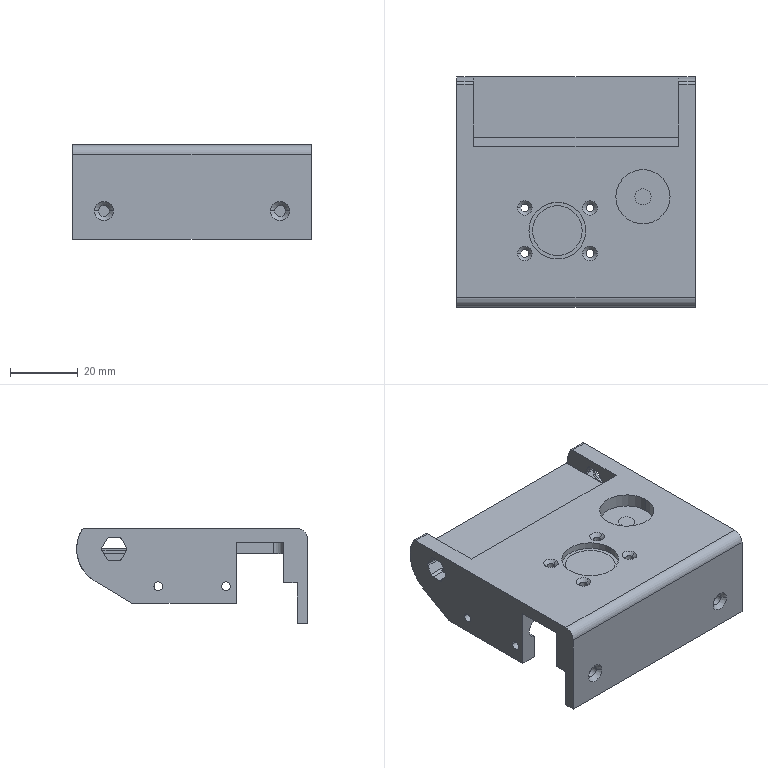NC program | NX | posted with a generic post | part box 70.5 x 68.1 x 28 mm
Lines 654 to 1476 of 2864:
(ZLEVEL_PROFILE_COPY_COPY_1 , TOOL : D2R0.5)
N1288 T09 M6
N1290 G54
N1292 G17 G0 G90 X57.923 Y-3.149 B0. C0. S9500 M3
N1294 G43 Z30. H9
N1296 Z1.
N1298 G94 G1 X57.717 Y-3.082 Z0.989 F1000.
N1300 X57.46 Y-3.043 Z0.975
N1302 X57.229 Y-3.004 Z0.963
N1304 X56.766 Z0.939
N1306 X56.526 Y-3.046 Z0.926
N1308 X56.302 Y-3.076 Z0.914
N1310 X56.048 Y-3.149 Z0.9
N1312 X55.841 Y-3.242 Z0.888
N1314 X55.642 Y-3.322 Z0.877
N1316 X55.312 Y-3.527 Z0.857
N1318 X55.164 Y-3.637 Z0.847
N1320 X55.005 Y-3.749 Z0.837
N1322 X54.966 Y-3.784 Z0.834
N1324 X54.829 Y-3.941 Z0.823
N1326 X54.661 Y-4.116 Z0.81
N1328 X54.308 Y-4.663 Z0.776
N1330 X54.084 Y-5.274 Z0.742
N1332 X54.045 Y-5.519 Z0.729
N1334 X54.027 Y-5.606 Z0.724
N1336 X54.001 Y-6.006 Z0.703
N1338 X54.027 Y-6.394 Z0.683
N1340 X54.046 Y-6.485 Z0.678
N1342 X54.083 Y-6.723 Z0.666
N1344 X54.285 Y-7.292 Z0.634
N1346 X54.601 Y-7.807 Z0.602
N1348 X54.948 Y-8.191 Z0.575
N1350 X55.13 Y-8.355 Z0.562
N1352 X55.236 Y-8.434 Z0.555
N1354 X55.447 Y-8.558 Z0.543
N1356 X55.688 Y-8.693 Z0.528
N1358 X55.9 Y-8.798 Z0.516
N1360 X56.291 Y-8.92 Z0.494
N1362 X56.54 Y-8.957 Z0.481
N1364 X56.771 Y-8.996 Z0.469
N1366 X57.234 Z0.444
N1368 X57.474 Y-8.954 Z0.432
N1370 X57.693 Y-8.926 Z0.42
N1372 X57.959 Y-8.85 Z0.406
N1374 X58.159 Y-8.758 Z0.394
N1376 X58.435 Y-8.629 Z0.378
N1378 X58.745 Y-8.442 Z0.359
N1380 X58.836 Y-8.364 Z0.353
N1382 X59.005 Y-8.24 Z0.342
N1384 X59.021 Y-8.225 Z0.341
N1386 X59.171 Y-8.059 Z0.329
N1388 X59.339 Y-7.884 Z0.316
N1390 X59.692 Y-7.337 Z0.282
N1392 X59.916 Y-6.726 Z0.248
N1394 X59.955 Y-6.481 Z0.235
N1396 X59.973 Y-6.394 Z0.23
N1398 X59.999 Y-6.006 Z0.21
N1400 X59.973 Y-5.606 Z0.189
N1402 X59.954 Y-5.515 Z0.184
N1404 X59.917 Y-5.277 Z0.172
N1406 X59.715 Y-4.708 Z0.14
N1408 X59.399 Y-4.193 Z0.108
N1410 X59.052 Y-3.809 Z0.081
N1412 X58.88 Y-3.651 Z0.069
N1414 X58.856 Y-3.633 Z0.067
N1416 X58.392 Y-3.341 Z0.039
N1418 X58.173 Y-3.229 Z0.026
N1420 X57.717 Y-3.082 Z0.001
N1422 X57.46 Y-3.043 Z-0.013
N1424 X57.229 Y-3.004 Z-0.025
N1426 X56.766 Z-0.05
N1428 X56.526 Y-3.046 Z-0.062
N1430 X56.302 Y-3.076 Z-0.074
N1432 X56.048 Y-3.149 Z-0.088
N1434 X55.841 Y-3.242 Z-0.1
N1436 X55.642 Y-3.322 F1500.
N1438 X55.312 Y-3.527
N1440 X55.164 Y-3.637
N1442 G3 X54.829 Y-3.941 R1.882
N1444 X54.045 Y-5.519 R2.943
N1446 G1 X54.027 Y-5.606
N1448 X54.001 Y-6.006
N1450 X54.027 Y-6.394
N1452 X54.046 Y-6.485
N1454 G3 X54.763 Y-7.986 R2.902
N1456 G1 X54.948 Y-8.191
N1458 G3 X55.447 Y-8.558 R2.996
N1460 G1 X55.688 Y-8.693
N1462 G3 X56.528 Y-8.954 R2.799
N1464 G1 X56.54 Y-8.957
N1466 G3 X57.474 Y-8.954 R2.743
N1468 X58.159 Y-8.758 R2.426
N1470 G1 X58.435 Y-8.629
N1472 X58.644 Y-8.503
N1474 G3 X58.836 Y-8.364 R1.367
N1476 X59.171 Y-8.059 R2.181
N1478 X59.955 Y-6.481 R2.943
N1480 G1 X59.973 Y-6.394
N1482 X59.999 Y-6.006
N1484 X59.973 Y-5.606
N1486 X59.954 Y-5.515
N1488 G3 X59.237 Y-4.014 R2.902
N1490 G1 X59.052 Y-3.809
N1492 G3 X58.658 Y-3.509 R2.717
N1494 G1 X58.392 Y-3.341
N1496 G3 X57.46 Y-3.043 R3.012
N1498 X56.526 Y-3.046 R2.743
N1500 X55.841 Y-3.242 R2.542
N1502 G1 X55.75 Y-3.281 Z-0.102
N1504 X55.66 Y-3.321 Z-0.103
N1506 X55.573 Y-3.367 Z-0.105
N1508 X55.489 Y-3.418 Z-0.107
N1510 X55.404 Y-3.469 Z-0.109
N1512 X55.32 Y-3.52 Z-0.11
N1514 X55.239 Y-3.577 Z-0.112
N1516 X55.161 Y-3.638 Z-0.114
N1518 X55.086 Y-3.702 Z-0.116
N1520 X55.009 Y-3.763 Z-0.117
N1522 X54.935 Y-3.829 Z-0.119
N1524 X54.867 Y-3.901 Z-0.121
N1526 X54.8 Y-3.973 Z-0.122
N1528 X54.732 Y-4.045 Z-0.124
N1530 X54.667 Y-4.119 Z-0.126
N1532 X54.609 Y-4.2 Z-0.128
N1534 X54.552 Y-4.28 Z-0.129
N1536 X54.496 Y-4.361 Z-0.131
N1538 X54.438 Y-4.442 Z-0.133
N1540 X54.393 Y-4.53 Z-0.134
N1542 X54.347 Y-4.617 Z-0.136
N1544 X54.302 Y-4.705 Z-0.138
N1546 X54.257 Y-4.793 Z-0.14
N1548 X54.222 Y-4.885 Z-0.141
N1550 X54.188 Y-4.978 Z-0.143
N1552 X54.155 Y-5.071 Z-0.145
N1554 X54.123 Y-5.164 Z-0.147
N1556 X54.099 Y-5.26 Z-0.148
N1558 X54.079 Y-5.357 Z-0.15
N1560 X54.059 Y-5.453 Z-0.152
N1562 X54.039 Y-5.55 Z-0.153
N1564 X54.026 Y-5.648 Z-0.155
N1566 X54.019 Y-5.746 Z-0.157
N1568 X54.013 Y-5.845 Z-0.159
N1570 X54.006 Y-5.943 Z-0.16
N1572 X54.003 Y-6.042 Z-0.162
N1574 X54.011 Y-6.14 Z-0.164
N1576 X54.018 Y-6.239 Z-0.166
N1578 X54.025 Y-6.337 Z-0.167
N1580 X54.035 Y-6.436 Z-0.169
N1582 X54.055 Y-6.532 Z-0.171
N1584 X54.076 Y-6.629 Z-0.172
N1586 X54.096 Y-6.725 Z-0.174
N1588 X54.117 Y-6.822 Z-0.176
N1590 X54.15 Y-6.915 Z-0.178
N1592 X54.184 Y-7.008 Z-0.179
N1594 X54.217 Y-7.101 Z-0.181
N1596 X54.25 Y-7.194 Z-0.183
N1598 X54.295 Y-7.282 Z-0.184
N1600 X54.341 Y-7.369 Z-0.186
N1602 X54.386 Y-7.457 Z-0.188
N1604 X54.431 Y-7.545 Z-0.19
N1606 X54.487 Y-7.627 Z-0.191
N1608 X54.544 Y-7.707 Z-0.193
N1610 X54.6 Y-7.788 Z-0.195
N1612 X54.658 Y-7.869 Z-0.197
N1614 X54.722 Y-7.943 Z-0.198
N1616 X54.79 Y-8.016 Z-0.2
N1618 X54.949 Y-8.191
N1620 G3 X55.447 Y-8.558 R2.994
N1622 G1 X55.688 Y-8.693
N1624 G3 X56.528 Y-8.954 R2.798
N1626 G1 X56.54 Y-8.957
N1628 G3 X57.474 Y-8.954 R2.743
N1630 X58.159 Y-8.758 R2.431
N1632 G1 X58.433 Y-8.63
N1634 X58.644 Y-8.503
N1636 G3 X58.836 Y-8.364 R1.367
N1638 X59.171 Y-8.059 R2.181
N1640 X59.955 Y-6.481 R2.943
N1642 G1 X59.973 Y-6.394
N1644 X59.999 Y-6.006
N1646 X59.973 Y-5.606
N1648 X59.954 Y-5.515
N1650 G3 X59.236 Y-4.013 R2.903
N1652 G1 X59.051 Y-3.809
N1654 G3 X58.659 Y-3.509 R2.714
N1656 G1 X58.392 Y-3.341
N1658 G3 X57.46 Y-3.043 R3.013
N1660 X56.526 Y-3.046 R2.743
N1662 X55.841 Y-3.242 R2.542
N1664 G1 X55.75 Y-3.281 Z-0.202
N1666 X55.66 Y-3.321 Z-0.203
N1668 X55.573 Y-3.367 Z-0.205
N1670 X55.489 Y-3.418 Z-0.207
N1672 X55.404 Y-3.469 Z-0.209
N1674 X55.32 Y-3.52 Z-0.21
N1676 X55.239 Y-3.577 Z-0.212
N1678 X55.161 Y-3.638 Z-0.214
N1680 X55.086 Y-3.701 Z-0.216
N1682 X55.009 Y-3.763 Z-0.217
N1684 X54.935 Y-3.829 Z-0.219
N1686 X54.867 Y-3.901 Z-0.221
N1688 X54.8 Y-3.973 Z-0.222
N1690 X54.732 Y-4.045 Z-0.224
N1692 X54.667 Y-4.119 Z-0.226
N1694 X54.609 Y-4.2 Z-0.228
N1696 X54.552 Y-4.28 Z-0.229
N1698 X54.496 Y-4.361 Z-0.231
N1700 X54.438 Y-4.442 Z-0.233
N1702 X54.393 Y-4.53 Z-0.234
N1704 X54.347 Y-4.617 Z-0.236
N1706 X54.302 Y-4.705 Z-0.238
N1708 X54.257 Y-4.793 Z-0.24
N1710 X54.222 Y-4.885 Z-0.241
N1712 X54.188 Y-4.978 Z-0.243
N1714 X54.155 Y-5.071 Z-0.245
N1716 X54.123 Y-5.164 Z-0.247
N1718 X54.099 Y-5.26 Z-0.248
N1720 X54.079 Y-5.357 Z-0.25
N1722 X54.059 Y-5.453 Z-0.252
N1724 X54.039 Y-5.55 Z-0.253
N1726 X54.026 Y-5.648 Z-0.255
N1728 X54.019 Y-5.746 Z-0.257
N1730 X54.013 Y-5.845 Z-0.259
N1732 X54.006 Y-5.943 Z-0.26
N1734 X54.003 Y-6.042 Z-0.262
N1736 X54.011 Y-6.14 Z-0.264
N1738 X54.018 Y-6.239 Z-0.266
N1740 X54.025 Y-6.337 Z-0.267
N1742 X54.035 Y-6.436 Z-0.269
N1744 X54.055 Y-6.532 Z-0.271
N1746 X54.076 Y-6.629 Z-0.272
N1748 X54.096 Y-6.725 Z-0.274
N1750 X54.117 Y-6.822 Z-0.276
N1752 X54.15 Y-6.915 Z-0.278
N1754 X54.184 Y-7.008 Z-0.279
N1756 X54.217 Y-7.101 Z-0.281
N1758 X54.25 Y-7.194 Z-0.283
N1760 X54.295 Y-7.282 Z-0.284
N1762 X54.34 Y-7.369 Z-0.286
N1764 X54.386 Y-7.457 Z-0.288
N1766 X54.431 Y-7.545 Z-0.29
N1768 X54.487 Y-7.627 Z-0.291
N1770 X54.544 Y-7.707 Z-0.293
N1772 X54.6 Y-7.788 Z-0.295
N1774 X54.658 Y-7.869 Z-0.297
N1776 X54.722 Y-7.943 Z-0.298
N1778 X54.79 Y-8.016 Z-0.3
N1780 X54.949 Y-8.191
N1782 G3 X55.447 Y-8.558 R2.993
N1784 G1 X55.689 Y-8.694
N1786 G3 X56.528 Y-8.954 R2.797
N1788 G1 X56.54 Y-8.957
N1790 G3 X57.474 Y-8.954 R2.743
N1792 X58.159 Y-8.758 R2.436
N1794 G1 X58.431 Y-8.631
N1796 X58.644 Y-8.503
N1798 G3 X58.836 Y-8.364 R1.367
N1800 X59.171 Y-8.059 R2.181
N1802 X59.955 Y-6.481 R2.943
N1804 G1 X59.973 Y-6.394
N1806 X59.999 Y-6.006
N1808 X59.973 Y-5.606
N1810 X59.954 Y-5.515
N1812 G3 X59.236 Y-4.012 R2.903
N1814 G1 X59.051 Y-3.809
N1816 G3 X58.659 Y-3.509 R2.712
N1818 G1 X58.392 Y-3.341
N1820 G3 X57.46 Y-3.043 R3.013
N1822 X56.526 Y-3.046 R2.743
N1824 X55.841 Y-3.242 R2.542
N1826 G1 X55.75 Y-3.281 Z-0.302
N1828 X55.66 Y-3.321 Z-0.303
N1830 X55.573 Y-3.367 Z-0.305
N1832 X55.489 Y-3.418 Z-0.307
N1834 X55.404 Y-3.469 Z-0.309
N1836 X55.32 Y-3.52 Z-0.31
N1838 X55.239 Y-3.577 Z-0.312
N1840 X55.161 Y-3.638 Z-0.314
N1842 X55.085 Y-3.701 Z-0.316
N1844 X55.009 Y-3.764 Z-0.317
N1846 X54.935 Y-3.829 Z-0.319
N1848 X54.867 Y-3.901 Z-0.321
N1850 X54.8 Y-3.973 Z-0.322
N1852 X54.732 Y-4.045 Z-0.324
N1854 X54.667 Y-4.119 Z-0.326
N1856 X54.609 Y-4.2 Z-0.328
N1858 X54.552 Y-4.28 Z-0.329
N1860 X54.496 Y-4.361 Z-0.331
N1862 X54.438 Y-4.442 Z-0.333
N1864 X54.393 Y-4.53 Z-0.334
N1866 X54.347 Y-4.617 Z-0.336
N1868 X54.302 Y-4.705 Z-0.338
N1870 X54.257 Y-4.793 Z-0.34
N1872 X54.222 Y-4.885 Z-0.341
N1874 X54.188 Y-4.978 Z-0.343
N1876 X54.155 Y-5.071 Z-0.345
N1878 X54.123 Y-5.164 Z-0.347
N1880 X54.099 Y-5.26 Z-0.348
N1882 X54.079 Y-5.357 Z-0.35
N1884 X54.059 Y-5.453 Z-0.352
N1886 X54.039 Y-5.55 Z-0.353
N1888 X54.026 Y-5.648 Z-0.355
N1890 X54.019 Y-5.746 Z-0.357
N1892 X54.013 Y-5.845 Z-0.359
N1894 X54.006 Y-5.943 Z-0.36
N1896 X54.003 Y-6.042 Z-0.362
N1898 X54.011 Y-6.14 Z-0.364
N1900 X54.018 Y-6.239 Z-0.366
N1902 X54.025 Y-6.337 Z-0.367
N1904 X54.035 Y-6.436 Z-0.369
N1906 X54.055 Y-6.532 Z-0.371
N1908 X54.076 Y-6.629 Z-0.372
N1910 X54.096 Y-6.725 Z-0.374
N1912 X54.117 Y-6.822 Z-0.376
N1914 X54.15 Y-6.915 Z-0.378
N1916 X54.184 Y-7.008 Z-0.379
N1918 X54.217 Y-7.101 Z-0.381
N1920 X54.25 Y-7.194 Z-0.383
N1922 X54.295 Y-7.282 Z-0.384
N1924 X54.34 Y-7.369 Z-0.386
N1926 X54.386 Y-7.457 Z-0.388
N1928 X54.431 Y-7.545 Z-0.39
N1930 X54.487 Y-7.627 Z-0.391
N1932 X54.544 Y-7.707 Z-0.393
N1934 X54.6 Y-7.788 Z-0.395
N1936 X54.658 Y-7.869 Z-0.397
N1938 X54.722 Y-7.943 Z-0.398
N1940 X54.79 Y-8.016 Z-0.4
N1942 X54.949 Y-8.191
N1944 G3 X55.447 Y-8.558 R2.991
N1946 G1 X55.689 Y-8.694
N1948 G3 X56.528 Y-8.954 R2.795
N1950 G1 X56.54 Y-8.957
N1952 G3 X57.474 Y-8.954 R2.743
N1954 X58.159 Y-8.758 R2.441
N1956 G1 X58.429 Y-8.632
N1958 X58.644 Y-8.503
N1960 G3 X58.836 Y-8.364 R1.367
N1962 X59.171 Y-8.059 R2.181
N1964 X59.955 Y-6.481 R2.943
N1966 G1 X59.973 Y-6.394
N1968 X59.999 Y-6.006
N1970 X59.973 Y-5.606
N1972 X59.954 Y-5.515
N1974 G3 X59.235 Y-4.012 R2.904
N1976 G1 X59.051 Y-3.809
N1978 G3 X58.659 Y-3.509 R2.71
N1980 G1 X58.392 Y-3.341
N1982 G3 X57.46 Y-3.043 R3.013
N1984 X56.526 Y-3.046 R2.743
N1986 X55.841 Y-3.242 R2.542
N1988 G1 X55.75 Y-3.281 Z-0.402
N1990 X55.66 Y-3.321 Z-0.403
N1992 X55.573 Y-3.367 Z-0.405
N1994 X55.489 Y-3.418 Z-0.407
N1996 X55.404 Y-3.469 Z-0.409
N1998 X55.32 Y-3.52 Z-0.41
N2000 X55.239 Y-3.577 Z-0.412
N2002 X55.162 Y-3.639 Z-0.414
N2004 X55.085 Y-3.701 Z-0.416
N2006 X55.009 Y-3.764 Z-0.417
N2008 X54.935 Y-3.829 Z-0.419
N2010 X54.867 Y-3.901 Z-0.421
N2012 X54.8 Y-3.973 Z-0.422
N2014 X54.733 Y-4.045 Z-0.424
N2016 X54.666 Y-4.119 Z-0.426
N2018 X54.61 Y-4.2 Z-0.428
N2020 X54.553 Y-4.28 Z-0.429
N2022 X54.496 Y-4.361 Z-0.431
N2024 X54.438 Y-4.442 Z-0.433
N2026 X54.393 Y-4.53 Z-0.434
N2028 X54.348 Y-4.617 Z-0.436
N2030 X54.303 Y-4.705 Z-0.438
N2032 X54.257 Y-4.793 Z-0.44
N2034 X54.221 Y-4.885 Z-0.441
N2036 X54.189 Y-4.978 Z-0.443
N2038 X54.156 Y-5.071 Z-0.445
N2040 X54.122 Y-5.164 Z-0.447
N2042 X54.099 Y-5.26 Z-0.448
N2044 X54.079 Y-5.357 Z-0.45
N2046 X54.059 Y-5.453 Z-0.452
N2048 X54.039 Y-5.55 Z-0.453
N2050 X54.026 Y-5.648 Z-0.455
N2052 X54.019 Y-5.746 Z-0.457
N2054 X54.013 Y-5.845 Z-0.459
N2056 X54.006 Y-5.943 Z-0.46
N2058 X54.004 Y-6.042 Z-0.462
N2060 X54.011 Y-6.14 Z-0.464
N2062 X54.017 Y-6.239 Z-0.466
N2064 X54.025 Y-6.337 Z-0.467
N2066 X54.036 Y-6.435 Z-0.469
N2068 X54.055 Y-6.532 Z-0.471
N2070 X54.076 Y-6.629 Z-0.472
N2072 X54.096 Y-6.725 Z-0.474
N2074 X54.117 Y-6.822 Z-0.476
N2076 X54.15 Y-6.915 Z-0.478
N2078 X54.184 Y-7.008 Z-0.479
N2080 X54.217 Y-7.101 Z-0.481
N2082 X54.25 Y-7.194 Z-0.483
N2084 X54.295 Y-7.282 Z-0.484
N2086 X54.341 Y-7.369 Z-0.486
N2088 X54.386 Y-7.457 Z-0.488
N2090 X54.431 Y-7.545 Z-0.49
N2092 X54.487 Y-7.626 Z-0.491
N2094 X54.544 Y-7.707 Z-0.493
N2096 X54.601 Y-7.788 Z-0.495
N2098 X54.658 Y-7.869 Z-0.497
N2100 X54.722 Y-7.944 Z-0.498
N2102 X54.783 Y-8.022 Z-0.5
N2104 G3 X55.838 Y-3.234 R-3.
N2106 G1 X55.747 Y-3.274 Z-0.502
N2108 X55.658 Y-3.317 Z-0.503
N2110 X55.571 Y-3.362 Z-0.505
N2112 X55.484 Y-3.411 Z-0.507
N2114 X55.4 Y-3.462 Z-0.509
N2116 X55.317 Y-3.516 Z-0.51
N2118 X55.237 Y-3.573 Z-0.512
N2120 X55.158 Y-3.632 Z-0.514
N2122 X55.081 Y-3.694 Z-0.516
N2124 X55.006 Y-3.759 Z-0.517
N2126 X54.933 Y-3.826 Z-0.519
N2128 X54.863 Y-3.895 Z-0.521
N2130 X54.795 Y-3.966 Z-0.522
N2132 X54.729 Y-4.04 Z-0.524
N2134 X54.665 Y-4.116 Z-0.526
N2136 X54.605 Y-4.194 Z-0.528
N2138 X54.547 Y-4.274 Z-0.529
N2140 X54.491 Y-4.355 Z-0.531
N2142 X54.438 Y-4.439 Z-0.533
N2144 X54.388 Y-4.524 Z-0.534
N2146 X54.341 Y-4.611 Z-0.536
N2148 X54.297 Y-4.699 Z-0.538
N2150 X54.255 Y-4.789 Z-0.54
N2152 X54.217 Y-4.88 Z-0.541
N2154 X54.182 Y-4.972 Z-0.543
N2156 X54.149 Y-5.065 Z-0.545
N2158 X54.12 Y-5.16 Z-0.547
N2160 X54.094 Y-5.255 Z-0.548
N2162 X54.071 Y-5.351 Z-0.55
N2164 X54.051 Y-5.448 Z-0.552
N2166 X54.035 Y-5.545 Z-0.553
N2168 X54.021 Y-5.643 Z-0.555
N2170 X54.011 Y-5.741 Z-0.557
N2172 X54.004 Y-5.84 Z-0.559
N2174 X54.001 Y-5.938 Z-0.56
N2176 X54. Y-6.037 Z-0.562
N2178 X54.003 Y-6.136 Z-0.564
N2180 X54.009 Y-6.234 Z-0.566
N2182 X54.019 Y-6.333 Z-0.567
N2184 X54.031 Y-6.431 Z-0.569
N2186 X54.047 Y-6.528 Z-0.571
N2188 X54.066 Y-6.625 Z-0.572
N2190 X54.088 Y-6.721 Z-0.574
N2192 X54.113 Y-6.817 Z-0.576
N2194 X54.142 Y-6.912 Z-0.578
N2196 X54.173 Y-7.005 Z-0.579
N2198 X54.208 Y-7.098 Z-0.581
N2200 X54.246 Y-7.189 Z-0.583
N2202 X54.286 Y-7.279 Z-0.584
N2204 X54.33 Y-7.368 Z-0.586
N2206 X54.376 Y-7.455 Z-0.588
N2208 X54.426 Y-7.54 Z-0.59
N2210 X54.478 Y-7.624 Z-0.591
N2212 X54.533 Y-7.706 Z-0.593
N2214 X54.59 Y-7.787 Z-0.595
N2216 X54.65 Y-7.865 Z-0.597
N2218 X54.713 Y-7.941 Z-0.598
N2220 X54.778 Y-8.016 Z-0.6
N2222 G3 X55.838 Y-3.234 R-3.
N2224 G1 X55.747 Y-3.274 Z-0.602
N2226 X55.658 Y-3.317 Z-0.603
N2228 X55.571 Y-3.362 Z-0.605
N2230 X55.484 Y-3.411 Z-0.607
N2232 X55.4 Y-3.462 Z-0.609
N2234 X55.317 Y-3.516 Z-0.61
N2236 X55.237 Y-3.573 Z-0.612
N2238 X55.158 Y-3.632 Z-0.614
N2240 X55.081 Y-3.694 Z-0.616
N2242 X55.006 Y-3.759 Z-0.617
N2244 X54.933 Y-3.826 Z-0.619
N2246 X54.863 Y-3.895 Z-0.621
N2248 X54.795 Y-3.966 Z-0.622
N2250 X54.729 Y-4.04 Z-0.624
N2252 X54.665 Y-4.116 Z-0.626
N2254 X54.605 Y-4.194 Z-0.628
N2256 X54.547 Y-4.274 Z-0.629
N2258 X54.491 Y-4.355 Z-0.631
N2260 X54.438 Y-4.439 Z-0.633
N2262 X54.388 Y-4.524 Z-0.634
N2264 X54.341 Y-4.611 Z-0.636
N2266 X54.297 Y-4.699 Z-0.638
N2268 X54.255 Y-4.789 Z-0.64
N2270 X54.217 Y-4.88 Z-0.641
N2272 X54.182 Y-4.972 Z-0.643
N2274 X54.149 Y-5.065 Z-0.645
N2276 X54.12 Y-5.16 Z-0.647
N2278 X54.094 Y-5.255 Z-0.648
N2280 X54.071 Y-5.351 Z-0.65
N2282 X54.051 Y-5.448 Z-0.652
N2284 X54.035 Y-5.545 Z-0.653
N2286 X54.021 Y-5.643 Z-0.655
N2288 X54.011 Y-5.741 Z-0.657
N2290 X54.004 Y-5.84 Z-0.659
N2292 X54.001 Y-5.938 Z-0.66
N2294 X54. Y-6.037 Z-0.662
N2296 X54.003 Y-6.136 Z-0.664
N2298 X54.009 Y-6.234 Z-0.666
N2300 X54.019 Y-6.333 Z-0.667
N2302 X54.031 Y-6.431 Z-0.669
N2304 X54.047 Y-6.528 Z-0.671
N2306 X54.066 Y-6.625 Z-0.672
N2308 X54.088 Y-6.721 Z-0.674
N2310 X54.113 Y-6.817 Z-0.676
N2312 X54.142 Y-6.912 Z-0.678
N2314 X54.173 Y-7.005 Z-0.679
N2316 X54.208 Y-7.098 Z-0.681
N2318 X54.246 Y-7.189 Z-0.683
N2320 X54.286 Y-7.279 Z-0.684
N2322 X54.33 Y-7.368 Z-0.686
N2324 X54.376 Y-7.455 Z-0.688
N2326 X54.426 Y-7.54 Z-0.69
N2328 X54.478 Y-7.624 Z-0.691
N2330 X54.533 Y-7.706 Z-0.693
N2332 X54.59 Y-7.787 Z-0.695
N2334 X54.65 Y-7.865 Z-0.697
N2336 X54.713 Y-7.941 Z-0.698
N2338 X54.778 Y-8.016 Z-0.7
N2340 G3 X55.838 Y-3.234 R-3.
N2342 G1 X55.747 Y-3.274 Z-0.702
N2344 X55.658 Y-3.317 Z-0.703
N2346 X55.571 Y-3.362 Z-0.705
N2348 X55.484 Y-3.411 Z-0.707
N2350 X55.4 Y-3.462 Z-0.709
N2352 X55.317 Y-3.516 Z-0.71
N2354 X55.237 Y-3.573 Z-0.712
N2356 X55.158 Y-3.632 Z-0.714
N2358 X55.081 Y-3.694 Z-0.716
N2360 X55.006 Y-3.759 Z-0.717
N2362 X54.933 Y-3.826 Z-0.719
N2364 X54.863 Y-3.895 Z-0.721
N2366 X54.795 Y-3.966 Z-0.722
N2368 X54.729 Y-4.04 Z-0.724
N2370 X54.665 Y-4.116 Z-0.726
N2372 X54.605 Y-4.194 Z-0.728
N2374 X54.547 Y-4.274 Z-0.729
N2376 X54.491 Y-4.355 Z-0.731
N2378 X54.438 Y-4.439 Z-0.733
N2380 X54.388 Y-4.524 Z-0.734
N2382 X54.341 Y-4.611 Z-0.736
N2384 X54.297 Y-4.699 Z-0.738
N2386 X54.255 Y-4.789 Z-0.74
N2388 X54.217 Y-4.88 Z-0.741
N2390 X54.182 Y-4.972 Z-0.743
N2392 X54.149 Y-5.065 Z-0.745
N2394 X54.12 Y-5.16 Z-0.747
N2396 X54.094 Y-5.255 Z-0.748
N2398 X54.071 Y-5.351 Z-0.75
N2400 X54.051 Y-5.448 Z-0.752
N2402 X54.035 Y-5.545 Z-0.753
N2404 X54.021 Y-5.643 Z-0.755
N2406 X54.011 Y-5.741 Z-0.757
N2408 X54.004 Y-5.84 Z-0.759
N2410 X54.001 Y-5.938 Z-0.76
N2412 X54. Y-6.037 Z-0.762
N2414 X54.003 Y-6.136 Z-0.764
N2416 X54.009 Y-6.234 Z-0.766
N2418 X54.019 Y-6.333 Z-0.767
N2420 X54.031 Y-6.431 Z-0.769
N2422 X54.047 Y-6.528 Z-0.771
N2424 X54.066 Y-6.625 Z-0.772
N2426 X54.088 Y-6.721 Z-0.774
N2428 X54.113 Y-6.817 Z-0.776
N2430 X54.142 Y-6.912 Z-0.778
N2432 X54.173 Y-7.005 Z-0.779
N2434 X54.208 Y-7.098 Z-0.781
N2436 X54.246 Y-7.189 Z-0.783
N2438 X54.286 Y-7.279 Z-0.784
N2440 X54.33 Y-7.368 Z-0.786
N2442 X54.376 Y-7.455 Z-0.788
N2444 X54.426 Y-7.54 Z-0.79
N2446 X54.478 Y-7.624 Z-0.791
N2448 X54.533 Y-7.706 Z-0.793
N2450 X54.59 Y-7.787 Z-0.795
N2452 X54.65 Y-7.865 Z-0.797
N2454 X54.713 Y-7.941 Z-0.798
N2456 X54.778 Y-8.016 Z-0.8
N2458 G3 X55.838 Y-3.234 R-3.
N2460 G1 X55.747 Y-3.274 Z-0.802
N2462 X55.658 Y-3.317 Z-0.803
N2464 X55.571 Y-3.362 Z-0.805
N2466 X55.484 Y-3.411 Z-0.807
N2468 X55.4 Y-3.462 Z-0.809
N2470 X55.317 Y-3.516 Z-0.81
N2472 X55.237 Y-3.573 Z-0.812
N2474 X55.158 Y-3.632 Z-0.814
N2476 X55.081 Y-3.694 Z-0.816
N2478 X55.006 Y-3.759 Z-0.817
N2480 X54.933 Y-3.826 Z-0.819
N2482 X54.863 Y-3.895 Z-0.821
N2484 X54.795 Y-3.966 Z-0.822
N2486 X54.729 Y-4.04 Z-0.824
N2488 X54.665 Y-4.116 Z-0.826
N2490 X54.605 Y-4.194 Z-0.828
N2492 X54.547 Y-4.274 Z-0.829
N2494 X54.491 Y-4.355 Z-0.831
N2496 X54.438 Y-4.439 Z-0.833
N2498 X54.388 Y-4.524 Z-0.834
N2500 X54.341 Y-4.611 Z-0.836
N2502 X54.297 Y-4.699 Z-0.838
N2504 X54.255 Y-4.789 Z-0.84
N2506 X54.217 Y-4.88 Z-0.841
N2508 X54.182 Y-4.972 Z-0.843
N2510 X54.149 Y-5.065 Z-0.845
N2512 X54.12 Y-5.16 Z-0.847
N2514 X54.094 Y-5.255 Z-0.848
N2516 X54.071 Y-5.351 Z-0.85
N2518 X54.051 Y-5.448 Z-0.852
N2520 X54.035 Y-5.545 Z-0.853
N2522 X54.021 Y-5.643 Z-0.855
N2524 X54.011 Y-5.741 Z-0.857
N2526 X54.004 Y-5.84 Z-0.859
N2528 X54.001 Y-5.938 Z-0.86
N2530 X54. Y-6.037 Z-0.862
N2532 X54.003 Y-6.136 Z-0.864
N2534 X54.009 Y-6.234 Z-0.866
N2536 X54.019 Y-6.333 Z-0.867
N2538 X54.031 Y-6.431 Z-0.869
N2540 X54.047 Y-6.528 Z-0.871
N2542 X54.066 Y-6.625 Z-0.872
N2544 X54.088 Y-6.721 Z-0.874
N2546 X54.113 Y-6.817 Z-0.876
N2548 X54.142 Y-6.912 Z-0.878
N2550 X54.173 Y-7.005 Z-0.879
N2552 X54.208 Y-7.098 Z-0.881
N2554 X54.246 Y-7.189 Z-0.883
N2556 X54.286 Y-7.279 Z-0.884
N2558 X54.33 Y-7.368 Z-0.886
N2560 X54.376 Y-7.455 Z-0.888
N2562 X54.426 Y-7.54 Z-0.89
N2564 X54.478 Y-7.624 Z-0.891
N2566 X54.533 Y-7.706 Z-0.893
N2568 X54.59 Y-7.787 Z-0.895
N2570 X54.65 Y-7.865 Z-0.897
N2572 X54.713 Y-7.941 Z-0.898
N2574 X54.778 Y-8.016 Z-0.9
N2576 G3 X55.838 Y-3.234 R-3.
N2578 G1 X55.747 Y-3.274 Z-0.902
N2580 X55.658 Y-3.317 Z-0.903
N2582 X55.571 Y-3.362 Z-0.905
N2584 X55.484 Y-3.411 Z-0.907
N2586 X55.4 Y-3.462 Z-0.909
N2588 X55.317 Y-3.516 Z-0.91
N2590 X55.237 Y-3.573 Z-0.912
N2592 X55.158 Y-3.632 Z-0.914
N2594 X55.081 Y-3.694 Z-0.916
N2596 X55.006 Y-3.759 Z-0.917
N2598 X54.933 Y-3.826 Z-0.919
N2600 X54.863 Y-3.895 Z-0.921
N2602 X54.795 Y-3.966 Z-0.922
N2604 X54.729 Y-4.04 Z-0.924
N2606 X54.665 Y-4.116 Z-0.926
N2608 X54.605 Y-4.194 Z-0.928
N2610 X54.547 Y-4.274 Z-0.929
N2612 X54.491 Y-4.355 Z-0.931
N2614 X54.438 Y-4.439 Z-0.933
N2616 X54.388 Y-4.524 Z-0.934
N2618 X54.341 Y-4.611 Z-0.936
N2620 X54.297 Y-4.699 Z-0.938
N2622 X54.255 Y-4.789 Z-0.94
N2624 X54.217 Y-4.88 Z-0.941
N2626 X54.182 Y-4.972 Z-0.943
N2628 X54.149 Y-5.065 Z-0.945
N2630 X54.12 Y-5.16 Z-0.947
N2632 X54.094 Y-5.255 Z-0.948
N2634 X54.071 Y-5.351 Z-0.95
N2636 X54.051 Y-5.448 Z-0.952
N2638 X54.035 Y-5.545 Z-0.953
N2640 X54.021 Y-5.643 Z-0.955
N2642 X54.011 Y-5.741 Z-0.957
N2644 X54.004 Y-5.84 Z-0.959
N2646 X54.001 Y-5.938 Z-0.96
N2648 X54. Y-6.037 Z-0.962
N2650 X54.003 Y-6.136 Z-0.964
N2652 X54.009 Y-6.234 Z-0.966
N2654 X54.019 Y-6.333 Z-0.967
N2656 X54.031 Y-6.431 Z-0.969
N2658 X54.047 Y-6.528 Z-0.971
N2660 X54.066 Y-6.625 Z-0.972
N2662 X54.088 Y-6.721 Z-0.974
N2664 X54.113 Y-6.817 Z-0.976
N2666 X54.142 Y-6.912 Z-0.978
N2668 X54.173 Y-7.005 Z-0.979
N2670 X54.208 Y-7.098 Z-0.981
N2672 X54.246 Y-7.189 Z-0.983
N2674 X54.286 Y-7.279 Z-0.984
N2676 X54.33 Y-7.368 Z-0.986
N2678 X54.376 Y-7.455 Z-0.988
N2680 X54.426 Y-7.54 Z-0.99
N2682 X54.478 Y-7.624 Z-0.991
N2684 X54.533 Y-7.706 Z-0.993
N2686 X54.59 Y-7.787 Z-0.995
N2688 X54.65 Y-7.865 Z-0.997
N2690 X54.713 Y-7.941 Z-0.998
N2692 X54.778 Y-8.016 Z-1.
N2694 G3 X55.838 Y-3.234 R-3.
N2696 G1 X55.747 Y-3.274 Z-1.002
N2698 X55.658 Y-3.317 Z-1.003
N2700 X55.571 Y-3.362 Z-1.005
N2702 X55.484 Y-3.411 Z-1.007
N2704 X55.4 Y-3.462 Z-1.009
N2706 X55.317 Y-3.516 Z-1.01
N2708 X55.237 Y-3.573 Z-1.012
N2710 X55.158 Y-3.632 Z-1.014
N2712 X55.081 Y-3.694 Z-1.016
N2714 X55.006 Y-3.759 Z-1.017
N2716 X54.933 Y-3.826 Z-1.019
N2718 X54.863 Y-3.895 Z-1.021
N2720 X54.795 Y-3.966 Z-1.022
N2722 X54.729 Y-4.04 Z-1.024
N2724 X54.665 Y-4.116 Z-1.026
N2726 X54.605 Y-4.194 Z-1.028
N2728 X54.547 Y-4.274 Z-1.029
N2730 X54.491 Y-4.355 Z-1.031
N2732 X54.438 Y-4.439 Z-1.033
N2734 X54.388 Y-4.524 Z-1.034
N2736 X54.341 Y-4.611 Z-1.036
N2738 X54.297 Y-4.699 Z-1.038
N2740 X54.255 Y-4.789 Z-1.04
N2742 X54.217 Y-4.88 Z-1.041
N2744 X54.182 Y-4.972 Z-1.043
N2746 X54.149 Y-5.065 Z-1.045
N2748 X54.12 Y-5.16 Z-1.047
N2750 X54.094 Y-5.255 Z-1.048
N2752 X54.071 Y-5.351 Z-1.05
N2754 X54.051 Y-5.448 Z-1.052
N2756 X54.035 Y-5.545 Z-1.053
N2758 X54.021 Y-5.643 Z-1.055
N2760 X54.011 Y-5.741 Z-1.057
N2762 X54.004 Y-5.84 Z-1.059
N2764 X54.001 Y-5.938 Z-1.06
N2766 X54. Y-6.037 Z-1.062
N2768 X54.003 Y-6.136 Z-1.064
N2770 X54.009 Y-6.234 Z-1.066
N2772 X54.019 Y-6.333 Z-1.067
N2774 X54.031 Y-6.431 Z-1.069
N2776 X54.047 Y-6.528 Z-1.071
N2778 X54.066 Y-6.625 Z-1.072
N2780 X54.088 Y-6.721 Z-1.074
N2782 X54.113 Y-6.817 Z-1.076
N2784 X54.142 Y-6.912 Z-1.078
N2786 X54.173 Y-7.005 Z-1.079
N2788 X54.208 Y-7.098 Z-1.081
N2790 X54.246 Y-7.189 Z-1.083
N2792 X54.286 Y-7.279 Z-1.084
N2794 X54.33 Y-7.368 Z-1.086
N2796 X54.376 Y-7.455 Z-1.088
N2798 X54.426 Y-7.54 Z-1.09
N2800 X54.478 Y-7.624 Z-1.091
N2802 X54.533 Y-7.706 Z-1.093
N2804 X54.59 Y-7.787 Z-1.095
N2806 X54.65 Y-7.865 Z-1.097
N2808 X54.713 Y-7.941 Z-1.098
N2810 X54.778 Y-8.016 Z-1.1
N2812 G3 X55.838 Y-3.234 R-3.
N2814 G1 X55.747 Y-3.274 Z-1.102
N2816 X55.658 Y-3.317 Z-1.103
N2818 X55.571 Y-3.362 Z-1.105
N2820 X55.484 Y-3.411 Z-1.107
N2822 X55.4 Y-3.462 Z-1.109
N2824 X55.317 Y-3.516 Z-1.11
N2826 X55.237 Y-3.573 Z-1.112
N2828 X55.158 Y-3.632 Z-1.114
N2830 X55.081 Y-3.694 Z-1.116
N2832 X55.006 Y-3.759 Z-1.117
N2834 X54.933 Y-3.826 Z-1.119
N2836 X54.863 Y-3.895 Z-1.121
N2838 X54.795 Y-3.966 Z-1.122
N2840 X54.729 Y-4.04 Z-1.124
N2842 X54.665 Y-4.116 Z-1.126
N2844 X54.605 Y-4.194 Z-1.128
N2846 X54.547 Y-4.274 Z-1.129
N2848 X54.491 Y-4.355 Z-1.131
N2850 X54.438 Y-4.439 Z-1.133
N2852 X54.388 Y-4.524 Z-1.134
N2854 X54.341 Y-4.611 Z-1.136
N2856 X54.297 Y-4.699 Z-1.138
N2858 X54.255 Y-4.789 Z-1.14
N2860 X54.217 Y-4.88 Z-1.141
N2862 X54.182 Y-4.972 Z-1.143
N2864 X54.149 Y-5.065 Z-1.145
N2866 X54.12 Y-5.16 Z-1.147
N2868 X54.094 Y-5.255 Z-1.148
N2870 X54.071 Y-5.351 Z-1.15
N2872 X54.051 Y-5.448 Z-1.152
N2874 X54.035 Y-5.545 Z-1.153
N2876 X54.021 Y-5.643 Z-1.155
N2878 X54.011 Y-5.741 Z-1.157
N2880 X54.004 Y-5.84 Z-1.159
N2882 X54.001 Y-5.938 Z-1.16
N2884 X54. Y-6.037 Z-1.162
N2886 X54.003 Y-6.136 Z-1.164
N2888 X54.009 Y-6.234 Z-1.166
N2890 X54.019 Y-6.333 Z-1.167
N2892 X54.031 Y-6.431 Z-1.169
N2894 X54.047 Y-6.528 Z-1.171
N2896 X54.066 Y-6.625 Z-1.172
N2898 X54.088 Y-6.721 Z-1.174
N2900 X54.113 Y-6.817 Z-1.176
N2902 X54.142 Y-6.912 Z-1.178
N2904 X54.173 Y-7.005 Z-1.179
N2906 X54.208 Y-7.098 Z-1.181
N2908 X54.246 Y-7.189 Z-1.183
N2910 X54.286 Y-7.279 Z-1.184
N2912 X54.33 Y-7.368 Z-1.186
N2914 X54.376 Y-7.455 Z-1.188
N2916 X54.426 Y-7.54 Z-1.19
N2918 X54.478 Y-7.624 Z-1.191
N2920 X54.533 Y-7.706 Z-1.193
N2922 X54.59 Y-7.787 Z-1.195
N2924 X54.65 Y-7.865 Z-1.197
N2926 X54.713 Y-7.941 Z-1.198